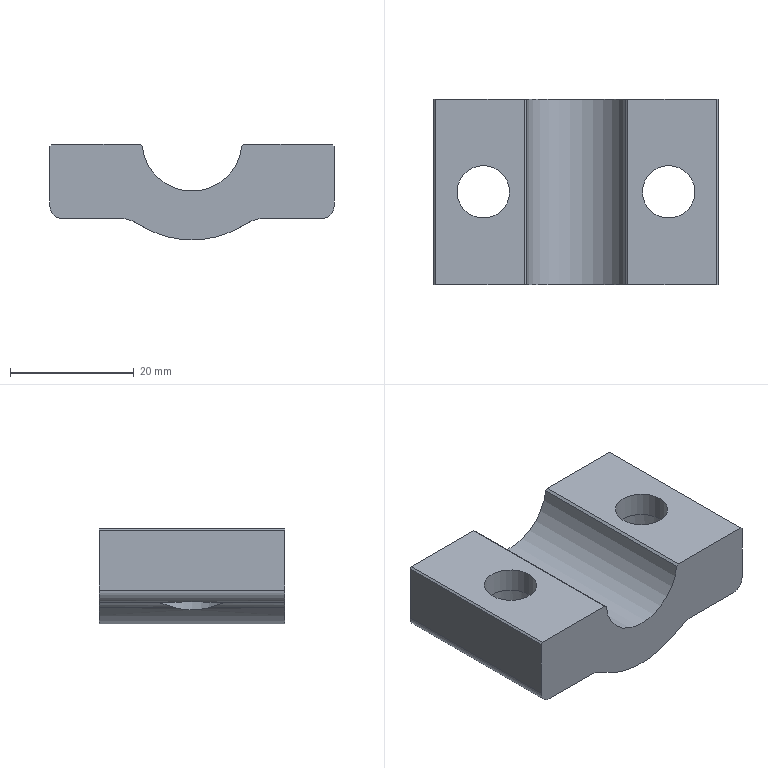NC program | NX | posted with a generic post | part box 46 x 30 x 15.5 mm
Lines 1 to 1684 of 1865, first 1555 of 1678 lines:
N10 G17 G21 G94 G90
(一刀光面 , TOOL : D50R6_1)
N12 T01 M6
N14 G54
N16 G17 G0 G90 X-52.998 Y-1.226 B0. C0. S2000 M3
N18 G43 Z30. H1
N20 Z3.
N22 G94 G1 Z0. F800.
N24 X-48. Y-1.08
N26 X48. Y1.739
N28 X52.998 Y1.886
N30 Z3.
N32 G0 Z30.
N34 M5
(ADAPTIVE_MILLING , TOOL : D10开粗_1)
N36 T02 M6
N38 G54
N40 G17 G0 G90 X-2.675 Y-20.135 B0. C0. S3000 M3
N42 G43 Z30. H2
N44 Z-28.
N46 G94 G1 X-2.599 Y-20.006 Z-28.937 F1500.
N48 X-2.522 Y-19.877 Z-29.308
N50 X-2.445 Y-19.748 Z-29.58
N52 X-2.369 Y-19.619 Z-29.8
N54 X-2.292 Y-19.49 Z-29.984
N56 X-2.216 Y-19.361 Z-30.142
N58 X-2.139 Y-19.232 Z-30.28
N60 X-2.063 Y-19.103 Z-30.4
N62 X-1.986 Y-18.974 Z-30.505
N64 X-1.91 Y-18.845 Z-30.598
N66 X-1.833 Y-18.716 Z-30.679
N68 X-1.757 Y-18.587 Z-30.75
N70 X-1.68 Y-18.458 Z-30.81
N72 X-1.604 Y-18.329 Z-30.862
N74 X-1.527 Y-18.2 Z-30.905
N76 X-1.451 Y-18.071 Z-30.939
N78 X-1.374 Y-17.942 Z-30.966
N80 X-1.298 Y-17.813 Z-30.985
N82 X-1.221 Y-17.684 Z-30.996
N84 X-1.145 Y-17.555 Z-31.
N86 X-0.452 Y-16.366
N88 G3 X-1.393 Y-14.946 R1.054
N90 X-5.461 Y-14.719 R28.472
N92 G1 X-23.555 Y-14.693
N94 G2 X-27.866 Y-12.146 R5.722
N96 X-29.421 Y-7.809 R9.762
N98 X-29.69 Y-2.044 R46.879
N100 G1 X-29.688 Y8.655
N102 G2 X-27.068 Y12.921 R5.762
N104 X-22.704 Y14.435 R9.932
N106 X-17.088 Y14.689 R48.084
N108 G1 X23.642 Y14.688
N110 G2 X27.877 Y12.131 R5.747
N112 X29.409 Y7.89 R9.699
N114 X29.686 Y2.539 R42.332
N116 X29.68 Y-8.741 R523.918
N118 X26.991 Y-12.972 R5.804
N120 X22.66 Y-14.441 R10.053
N122 X17.006 Y-14.69 R49.412
N124 G1 X0.569 Y-14.692
N126 G3 X-11.106 Y-14.4 R163.168
N128 G2 X-22.167 Y-14.38 R687.333
N130 X-27.657 Y-10.843 R6.986
N132 X-29.116 Y-6.184 R11.92
N134 X-29.391 Y0.294 R57.694
N136 X-29.38 Y7.166 R327.722
N138 X-25.778 Y12.695 R6.998
N140 X-20.997 Y14.138 R12.202
N142 X-14.706 Y14.391 R60.559
N144 G1 X21.829 Y14.396
N146 G2 X27.656 Y10.844 R6.967
N148 X29.115 Y6.184 R11.92
N150 X29.388 Y0.156 R54.035
N152 X29.38 Y-7.166 R332.394
N154 X25.811 Y-12.676 R6.993
N156 X21.184 Y-14.116 R11.962
N158 X14.856 Y-14.39 R56.43
N160 X0.746 Y-14.37 R762.628
N162 G3 X-11.706 Y-14.1 R214.037
N164 G2 X-20.854 Y-14.08 R721.079
N166 X-27.421 Y-9.795 R7.821
N168 X-28.832 Y-4.768 R13.795
N170 X-29.09 Y1.824 R66.58
N172 X-29.056 Y6.173 R66.922
N174 X-26.433 Y11.301 R7.585
N176 G1 X-26.341 Y11.392
N178 X-25.56 Y12.033
N180 G2 X-20.593 Y13.734 R12.355
N182 X-14.42 Y14.08 R48.356
N184 G1 X-9.433 Y14.099
N186 X20.142 Y14.098
N188 G2 X26.365 Y11.368 R7.784
N190 G1 X26.642 Y11.091
N192 X27.283 Y10.31
N194 X27.758 Y9.419
N196 G2 X28.907 Y4.167 R16.901
N198 X29.098 Y-4.116 R114.084
N200 X28.917 Y-7.104 R14.147
N202 X24.671 Y-12.486 R7.89
N204 X19.744 Y-13.835 R13.983
N206 X12.89 Y-14.092 R69.499
N208 X0.99 Y-14.06 R533.296
N210 G3 X-15.676 Y-13.798 R347.698
N212 G2 X-20.1 Y-13.754 R73.458
N214 X-27.142 Y-8.934 R8.455
N216 X-28.529 Y-3.707 R15.147
N218 X-28.753 Y5.06 R74.456
N220 X-28.115 Y7.864 R10.459
N222 G1 X-28.1 Y7.957
N224 X-28.051 Y8.456
N226 G2 X-27.281 Y10.312 R5.993
N228 X-26.429 Y11.304 R11.794
N230 G1 X-26.341 Y11.392
N232 X-25.56 Y12.033
N234 X-24.669 Y12.508
N236 X-23.703 Y12.801
N238 G2 X-15.324 Y13.747 R39.034
N240 X-6.737 Y13.799 R327.037
N242 G1 X18.701 Y13.798
N244 G2 X23.432 Y12.845 R10.105
N246 G1 X23.612 Y12.81
N248 G2 X24.672 Y12.507 R12.961
N250 X26.369 Y11.365 R5.971
N252 G3 X27.787 Y11.368 R1.003
N254 X27.787 Y12.782 R1.003
N256 G1 X26.533 Y14.326 Z-30.9
N258 X25.689 Y15.364 F15000.
N260 X25.589 Y15.471
N262 X25.474 Y15.561
N264 X25.347 Y15.634
N266 X25.21 Y15.688
N268 X24.023 Y16.057
N270 X23.547 Y16.197
N272 X23.066 Y16.321
N274 X22.582 Y16.43
N276 X22.094 Y16.522
N278 X21.604 Y16.599
N280 X20.988 Y16.675
N282 X20.37 Y16.728
N284 X19.75 Y16.76
N286 X19.13 Y16.769
N288 X-21.465 Y16.678
N290 X-21.6 Y16.668
N292 X-21.732 Y16.641
N294 X-21.859 Y16.596
N296 X-21.979 Y16.534
N298 X-22.09 Y16.457
N300 X-23.487 Y15.333
N302 X-24.524 Y14.488 Z-30.967 F1500.
N304 X-24.678 Y14.278 Z-30.98
N306 X-24.772 Y14.036 Z-30.993
N308 X-24.795 Y13.908 Z-31.
N310 X-24.801 Y13.76
N312 G3 X-23.703 Y12.801 R1.
N314 G1 X-22.699 Y12.9
N316 G2 X-16.524 Y13.388 R122.432
N318 X-6.626 Y13.499 R238.027
N320 G1 X17.479 Y13.498
N322 G2 X22.03 Y12.91 R15.267
N324 G1 X22.163 Y12.9
N326 X22.701
N328 X23.634 Y12.808
N330 G3 X24.702 Y14.047 R1.
N332 G1 X24.591 Y14.315 Z-30.985
N334 X24.407 Y14.54 Z-30.971
N336 X23.249 Y15.339 Z-30.9
N338 X22.235 Y16.027 F15000.
N340 X22.106 Y16.101
N342 X21.968 Y16.155
N344 X21.823 Y16.188
N346 X21.675 Y16.2
N348 X-20.741 Y16.292
N350 X-20.865 Y16.284
N352 X-20.987 Y16.262
N354 X-21.105 Y16.224
N356 X-21.218 Y16.172
N358 X-21.323 Y16.107
N360 X-22.321 Y15.396
N362 X-23.384 Y14.629 Z-30.966 F1500.
N364 X-23.554 Y14.419 Z-30.98
N366 X-23.662 Y14.171 Z-30.993
N368 X-23.69 Y14.038 Z-31.
N370 X-23.699 Y13.896
N372 G3 X-22.699 Y12.9 R1.
N374 G1 X-20.787
N376 G2 X-5.133 Y13.198 R277.211
N378 G1 X16.242
N380 G2 X20.329 Y12.9 R22.152
N382 G1 X22.167
N384 G3 X22.48 Y14.85 R1.
N386 G1 X20.563 Y15.383 Z-30.9
N388 X19.665 Y15.633 F15000.
N390 X19.533 Y15.66
N392 X19.397 Y15.669
N394 X-18.017
N396 X-18.152 Y15.66
N398 X-18.285 Y15.633
N400 X-19.158 Y15.39
N402 X-21.075 Y14.858 Z-31. F1500.
N404 G3 X-20.787 Y12.9 R1.
N406 G1 X-8.389
N408 X8.386
N410 X8.391
N412 X20.353
N414 G3 X21.453 Y14. R1.1
N416 X20.353 Y15.1 R1.1
N418 G1 X8.393 Y15.098
N420 X6.403 Z-30.9
N422 X-6.368 Y15.096 F15000.
N424 X-8.357 Y15.093 Z-31. F1500.
N426 G3 X-8.389 Y12.9 R1.1
N428 G1 X-7.446 Y12.813
N430 G3 X-2.884 Y12.611 R38.96
N432 X6.716 Y12.613 R688.468
N434 G1 X6.832 Y12.639
N436 X7.449 Y12.813
N438 X8.391 Y12.9
N440 G3 X8.328 Y15.095 R1.1
N442 G1 X6.338 Y15.08 Z-30.9
N444 X-5.963 Y14.981 F15000.
N446 X-7.314 Y14.958 Z-30.968 F1500.
N448 X-7.618 Y14.865 Z-30.984
N450 X-7.882 Y14.689 Z-31.
N452 G3 X-7.446 Y12.813 R1.1
N454 G1 X-7.014 Y12.69
N456 G3 X-3.381 Y12.353 R19.2
N458 X5.761 Y12.316 R248.059
N460 X6.292 Y12.433 R1.24
N462 G1 X6.539 Y12.556
N464 X6.863 Y12.647
N466 G3 X7.393 Y14.429 R1.1
N468 G1 X7.158 Y14.632 Z-30.984
N470 X6.875 Y14.761 Z-30.969
N472 X6.567 Y14.806 Z-30.953
N474 X5.514 Y14.809 Z-30.9
N476 X-5.579 Y14.845 F15000.
N478 X-6.853 Y14.839 Z-30.964 F1500.
N480 X-7.129 Y14.767 Z-30.978
N482 X-7.377 Y14.626 Z-30.993
N484 X-7.485 Y14.532 Z-31.
N486 X-7.586 Y14.418
N488 G3 X-7.014 Y12.69 R1.1
N490 G1 X-6.536 Y12.555
N492 G3 X-3.407 Y12.111 R12.813
N494 X5.064 Y12.033 R126.648
N496 X5.763 Y12.171 R1.657
N498 G1 X6.301 Y12.438
N500 G3 X6.746 Y14.006 R1.1
N502 G1 X6.543 Y14.246 Z-30.984
N504 X6.281 Y14.419 Z-30.968
N506 X5.98 Y14.511 Z-30.952
N508 X4.937 Y14.532 Z-30.9
N510 X-5.115 Y14.631 F15000.
N512 X-6.189 Z-30.954 F1500.
N514 X-6.482 Y14.551 Z-30.969
N516 X-6.742 Y14.393 Z-30.985
N518 X-6.949 Y14.17 Z-31.
N520 G3 X-6.536 Y12.555 R1.1
N522 G1 X-6.301 Y12.438
N524 G3 X-3.478 Y11.89 R9.865
N526 X4.495 Y11.754 R77.735
N528 X5.549 Y12.03 R2.077
N530 G1 X5.691 Y12.136
N532 X5.791 Y12.186
N534 G3 X6.262 Y13.711 R1.1
N536 G1 X6.092 Y13.938 Z-30.986
N538 X5.869 Y14.115 Z-30.971
N540 X5.609 Y14.228 Z-30.957
N542 X5.328 Y14.271 Z-30.943
N544 X4.478 Y14.29 Z-30.9
N546 X-4.856 Y14.502 F15000.
N548 X-5.938 Y14.516 Z-30.954 F1500.
N550 X-6.23 Y14.441 Z-30.97
N552 X-6.49 Y14.29 Z-30.985
N554 X-6.7 Y14.073 Z-31.
N556 G3 X-6.301 Y12.438 R1.1
N558 G1 X-5.898 Y12.238
N560 G3 X-2.979 Y11.627 R10.034
N562 X4.013 Y11.481 R53.438
N564 X5.215 Y11.781 R2.627
N566 G1 X5.251 Y11.806
N568 X5.551 Y12.031
N570 G3 X5.861 Y13.428 R1.1
N572 G1 X5.693 Y13.663 Z-30.985
N574 X5.471 Y13.845 Z-30.971
N576 X5.208 Y13.964 Z-30.956
N578 X4.924 Y14.01 Z-30.942
N580 X4.09 Y14.035 Z-30.9
N582 X-4.465 Y14.295 F15000.
N584 X-5.53 Y14.317 Z-30.954 F1500.
N586 X-5.827 Y14.241 Z-30.969
N588 X-6.092 Y14.086 Z-30.985
N590 X-6.304 Y13.863 Z-31.
N592 G3 X-5.898 Y12.238 R1.1
N594 G1 X-5.688 Y12.134
N596 G3 X-3.356 Y11.468 R6.927
N598 X3.607 Y11.215 R37.805
N600 X4.884 Y11.532 R2.908
N602 G1 X4.933 Y11.567
N604 X5.263 Y11.815
N606 G3 X5.575 Y13.21 R1.1
N608 G1 X5.408 Y13.445 Z-30.985
N610 X5.186 Y13.628 Z-30.971
N612 X4.924 Y13.747 Z-30.956
N614 X4.64 Y13.794 Z-30.942
N616 X3.806 Y13.822 Z-30.9
N618 X-4.134 Y14.085 F15000.
N620 X-5.153 Y14.107 Z-30.951 F1500.
N622 X-5.464 Y14.024 Z-30.967
N624 X-5.738 Y13.854 Z-30.984
N626 X-5.951 Y13.612 Z-31.
N628 G3 X-5.688 Y12.134 R1.1
N630 G1 X-5.538 Y12.022
N632 G3 X-3.196 Y11.252 R6.403
N634 X3.384 Y10.97 R28.714
N636 X4.667 Y11.334 R2.802
N638 G1 X4.743 Y11.395
N640 X4.933 Y11.567
N642 X4.963 Y11.59
N644 G3 X5.281 Y12.972 R1.1
N646 G1 X5.118 Y13.209 Z-30.986
N648 X4.898 Y13.395 Z-30.971
N650 X4.638 Y13.517 Z-30.957
N652 X4.355 Y13.568 Z-30.942
N654 X3.52 Y13.608 Z-30.9
N656 X-3.968 Y13.96 F15000.
N658 X-4.987 Y13.996 Z-30.951 F1500.
N660 X-5.3 Y13.917 Z-30.968
N662 X-5.576 Y13.752 Z-30.984
N664 X-5.792 Y13.513 Z-31.
N666 G3 X-5.538 Y12.022 R1.1
N668 G1 X-5.268 Y11.819
N670 G3 X-2.768 Y10.985 R6.955
N672 X3.117 Y10.725 R23.466
N674 X4.416 Y11.098 R3.059
N676 G1 X4.576 Y11.239
N678 X4.604 Y11.269
N680 X4.77 Y11.42
N682 G3 X5.006 Y12.747 R1.1
N684 G1 X4.815 Y13.008 Z-30.984
N686 X4.556 Y13.202 Z-30.967
N688 X4.252 Y13.313 Z-30.951
N690 X3.239 Y13.379 Z-30.9
N692 X-3.691 Y13.751 F15000.
N694 X-4.71 Y13.794 Z-30.951 F1500.
N696 X-5.023 Y13.717 Z-30.968
N698 X-5.3 Y13.554 Z-30.984
N700 X-5.518 Y13.317 Z-31.
N702 G3 X-5.268 Y11.819 R1.1
N704 G1 X-4.999 Y11.616
N706 G3 X-2.544 Y10.75 R6.898
N708 X2.956 Y10.497 R19.039
N710 X4.263 Y10.918 R2.878
N712 G1 X4.382 Y11.027
N714 X4.585 Y11.248
N716 G3 X4.747 Y12.506 R1.1
N718 G1 X4.558 Y12.764 Z-30.984
N720 X4.302 Y12.957 Z-30.968
N722 X4.002 Y13.069 Z-30.952
N724 X2.981 Y13.144 Z-30.9
N726 X-3.412 Y13.541 F15000.
N728 X-4.431 Y13.592 Z-30.951 F1500.
N730 X-4.744 Y13.518 Z-30.968
N732 X-5.022 Y13.357 Z-30.984
N734 X-5.242 Y13.122 Z-31.
N736 G3 X-4.999 Y11.616 R1.1
N738 G1 X-4.932 Y11.566
N740 X-4.849 Y11.491
N742 G3 X-2.567 Y10.567 R5.905
N744 X2.79 Y10.274 R16.159
N746 X4.075 Y10.709 R2.832
N748 G1 X4.179 Y10.807
N750 X4.382 Y11.028
N752 G3 X4.538 Y12.297 R1.1
N754 G1 X4.35 Y12.549 Z-30.984
N756 X4.099 Y12.738 Z-30.968
N758 X3.804 Y12.847 Z-30.952
N760 X2.765 Y12.931 Z-30.9
N762 X-3.181 Y13.344 F15000.
N764 X-4.196 Y13.403 Z-30.951 F1500.
N766 X-4.511 Y13.331 Z-30.967
N768 X-4.791 Y13.17 Z-30.984
N770 X-5.012 Y12.935 Z-31.
N772 G3 X-4.849 Y11.491 R1.1
N774 G1 X-4.626 Y11.289
N776 G3 X-2.23 Y10.306 R6.145
N778 X2.794 Y10.086 R13.405
N780 X3.946 Y10.555 R2.253
N782 G1 X3.98 Y10.59
N784 X4.183 Y10.811
N786 G3 X4.341 Y12.077 R1.1
N788 G1 X4.155 Y12.329 Z-30.984
N790 X3.905 Y12.518 Z-30.968
N792 X3.612 Y12.629 Z-30.953
N794 X2.57 Y12.719 Z-30.9
N796 X-2.952 Y13.137 F15000.
N798 X-3.967 Y13.202 Z-30.951 F1500.
N800 X-4.282 Y13.132 Z-30.967
N802 X-4.563 Y12.973 Z-30.984
N804 X-4.786 Y12.739 Z-31.
N806 G3 X-4.527 Y11.185 R1.158
N808 X-2.363 Y10.159 R5.259
N810 X2.666 Y9.88 R11.9
N812 X3.824 Y10.389 R2.204
N814 X4.274 Y11.278 R1.578
N816 X4.148 Y11.857 R1.1
N818 G1 X3.963 Y12.109 Z-30.984
N820 X3.716 Y12.299 Z-30.969
N822 X3.424 Y12.412 Z-30.953
N824 X2.381 Y12.512 Z-30.9
N826 X-2.763 Y12.951 F15000.
N828 X-3.783 Y13.027 Z-30.951 F1500.
N830 X-4.097 Y12.961 Z-30.968
N832 X-4.379 Y12.807 Z-30.984
N834 X-4.604 Y12.578 Z-31.
N836 G3 X-4.527 Y11.185 R1.1
N838 G1 X-4.374 Y11.019
N840 G3 X-2.25 Y9.954 R5.158
N842 X2.604 Y9.694 R10.483
N844 X3.744 Y10.246 R2.135
N846 G1 X3.837 Y10.369
N848 X3.956 Y10.56
N850 G3 X3.984 Y11.68 R1.1
N852 G1 X3.801 Y11.922 Z-30.985
N854 X3.559 Y12.104 Z-30.969
N856 X3.277 Y12.214 Z-30.954
N858 X2.206 Y12.325 Z-30.9
N860 X-2.606 Y12.778 F15000.
N862 X-3.622 Y12.861 Z-30.951 F1500.
N864 X-3.938 Y12.797 Z-30.968
N866 X-4.221 Y12.645 Z-30.984
N868 X-4.448 Y12.417 Z-31.
N870 G3 X-4.374 Y11.019 R1.1
N872 G1 X-4.172 Y10.798
N874 G3 X-1.881 Y9.679 R5.381
N876 X2.528 Y9.51 R9.392
N878 X3.664 Y10.106 R2.044
N880 G1 X3.725 Y10.191
N882 X3.845 Y10.382
N884 G3 X3.855 Y11.531 R1.1
N886 G1 X3.672 Y11.761 Z-30.985
N888 X3.434 Y11.934 Z-30.97
N890 X3.158 Y12.037 Z-30.956
N892 X2.06 Y12.148 Z-30.9
N894 X-2.405 Y12.559 F15000.
N896 X-3.422 Y12.64 Z-30.951 F1500.
N898 X-3.737 Y12.576 Z-30.968
N900 X-4.02 Y12.423 Z-30.984
N902 X-4.247 Y12.194 Z-31.
N904 G3 X-4.172 Y10.798 R1.1
N906 G1 X-3.962 Y10.57
N908 G3 X-1.6 Y9.431 R5.475
N910 X2.558 Y9.36 R8.289
N912 X3.608 Y10.004 R1.785
N914 G1 X3.728 Y10.194
N916 G3 X3.716 Y11.379 R1.1
N918 G1 X3.526 Y11.599 Z-30.985
N920 X3.285 Y11.762 Z-30.971
N922 X3.01 Y11.857 Z-30.956
N924 X1.899 Y11.937 Z-30.9
N926 X-2.076 Y12.191 F15000.
N928 X-3.115 Y12.246 Z-30.952 F1500.
N930 X-3.422 Y12.176 Z-30.968
N932 X-3.697 Y12.022 Z-30.984
N934 X-3.917 Y11.796 Z-31.
N936 G3 X-3.617 Y10.212 R1.114
N938 X-0.637 Y9.054 R6.462
N940 X2.699 Y9.258 R6.944
N942 X3.491 Y9.816 R1.395
N944 G1 X3.61 Y10.006
N946 G3 X3.605 Y11.181 R1.1
N948 G1 X3.423 Y11.399 Z-30.986
N950 X3.191 Y11.562 Z-30.971
N952 X2.926 Y11.661 Z-30.957
N954 X1.796 Y11.782 Z-30.9
N956 X-2.055 Y12.162 F15000.
N958 X-3.081 Y12.252 Z-30.952 F1500.
N960 X-3.394 Y12.191 Z-30.968
N962 X-3.676 Y12.043 Z-30.984
N964 X-3.904 Y11.821 Z-31.
N966 G3 X-3.962 Y10.57 R1.1
N968 G1 X-3.863 Y10.411
N970 G3 X-1.993 Y9.222 R4.072
N972 X2.42 Y9.014 R7.269
N974 X3.574 Y9.97 R1.638
N976 X3.496 Y11.002 R1.1
N978 G1 X3.316 Y11.219 Z-30.986
N980 X3.086 Y11.383 Z-30.972
N982 X2.822 Y11.483 Z-30.957
N984 X1.689 Y11.612 Z-30.9
N986 X-1.927 Y11.994 F15000.
N988 X-2.971 Y12.093 Z-30.953 F1500.
N990 X-3.278 Y12.037 Z-30.968
N992 X-3.558 Y11.897 Z-30.984
N994 X-3.786 Y11.684 Z-31.
N996 G3 X-3.863 Y10.411 R1.1
N998 G1 X-3.764 Y10.252
N1000 G3 X-1.914 Y9.039 R4.047
N1002 X2.313 Y8.833 R6.919
N1004 X3.354 Y9.528 R1.746
N1006 X3.362 Y10.771 R1.169
N1008 G1 X3.152 Y11.01 Z-30.984
N1010 X2.882 Y11.179 Z-30.968
N1012 X2.576 Y11.264 Z-30.952
N1014 X1.552 Y11.393 Z-30.9
N1016 X-1.8 Y11.814 F15000.
N1018 X-2.849 Y11.935 Z-30.953 F1500.
N1020 X-3.155 Y11.886 Z-30.969
N1022 X-3.436 Y11.754 Z-30.984
N1024 X-3.668 Y11.548 Z-31.
N1026 G3 X-3.764 Y10.252 R1.1
N1028 G1 X-3.664 Y10.093
N1030 G3 X-1.799 Y8.846 R3.942
N1032 X2.248 Y8.668 R6.552
N1034 X3.294 Y9.376 R1.801
N1036 G1 X3.359 Y9.509
N1038 X3.428 Y9.683
N1040 G3 X3.314 Y10.704 R1.1
N1042 G1 X3.102 Y10.936 Z-30.984
N1044 X2.834 Y11.099 Z-30.968
N1046 X2.53 Y11.179 Z-30.952
N1048 X1.493 Y11.298 Z-30.9
N1050 X-1.707 Y11.666 F15000.
N1052 X-2.761 Y11.776 Z-30.953 F1500.
N1054 X-3.065 Y11.724 Z-30.969
N1056 X-3.344 Y11.59 Z-30.984
N1058 X-3.574 Y11.384 Z-31.
N1060 G3 X-3.664 Y10.093 R1.1
N1062 G1 X-3.545 Y9.902
N1064 G3 X-1.65 Y8.643 R3.964
N1066 X2.239 Y8.524 R6.144
N1068 X3.249 Y9.249 R1.738
N1070 G1 X3.3 Y9.358
N1072 X3.369 Y9.533
N1074 G3 X3.235 Y10.582 R1.1
N1076 G1 X3.024 Y10.801 Z-30.985
N1078 X2.761 Y10.954 Z-30.969
N1080 X2.466 Y11.029 Z-30.954
N1082 X1.399 Y11.147 Z-30.9
N1084 X-1.59 Y11.479 F15000.
N1086 X-2.645 Y11.585 Z-30.953 F1500.
N1088 X-2.949 Y11.532 Z-30.969
N1090 X-3.227 Y11.397 Z-30.984
N1092 X-3.456 Y11.191 Z-31.
N1094 G3 X-3.545 Y9.902 R1.1
N1096 G1 X-3.461 Y9.768
N1098 G3 X-1.724 Y8.524 R3.589
N1100 X2.338 Y8.427 R5.681
N1102 X3.237 Y9.197 R1.514
N1104 G1 X3.305 Y9.371
N1106 G3 X3.151 Y10.449 R1.1
N1108 G1 X2.934 Y10.66 Z-30.985
N1110 X2.669 Y10.804 Z-30.97
N1112 X2.374 Y10.87 Z-30.954
N1114 X1.298 Y10.96 Z-30.9
N1116 X-1.408 Y11.187 F15000.
N1118 X-2.495 Y11.268 Z-30.955 F1500.
N1120 X-2.788 Y11.212 Z-30.97
N1122 X-3.056 Y11.079 Z-30.985
N1124 X-3.278 Y10.879 Z-31.
N1126 G3 X-3.082 Y9.238 R1.175
N1128 X0.036 Y7.967 R5.119
N1130 X2.637 Y8.451 R4.489
N1132 X3.174 Y9.037 R1.168
N1134 G1 X3.242 Y9.212
N1136 G3 X3.084 Y10.293 R1.1
N1138 G1 X2.877 Y10.496 Z-30.985
N1140 X2.623 Y10.637 Z-30.971
N1142 X2.341 Y10.707 Z-30.956
N1144 X1.233 Y10.832 Z-30.9
N1146 X-1.369 Y11.124 F15000.
N1148 X-2.451 Y11.235 Z-30.955 F1500.
N1150 X-2.746 Y11.187 Z-30.97
N1152 X-3.018 Y11.061 Z-30.985
N1154 X-3.246 Y10.866 Z-31.
N1156 G3 X-3.151 Y9.229 R1.221
N1158 X-0.576 Y7.897 R4.532
N1160 X2.452 Y8.222 R4.845
N1162 X3.115 Y8.887 R1.24
N1164 G1 X3.183 Y9.061
N1166 G3 X3.017 Y10.153 R1.1
N1168 G1 X2.812 Y10.35 Z-30.986
N1170 X2.563 Y10.487 Z-30.971
N1172 X2.288 Y10.556 Z-30.957
N1174 X1.16 Y10.689 Z-30.9
N1176 X-1.29 Y10.976 F15000.
N1178 X-2.388 Y11.095 Z-30.956 F1500.
N1180 X-2.678 Y11.051 Z-30.97
N1182 X-2.947 Y10.931 Z-30.985
N1184 X-3.174 Y10.745 Z-31.
N1186 G3 X-3.189 Y9.203 R1.197
N1188 X-0.822 Y7.802 R4.112
N1190 X2.356 Y8.048 R4.82
N1192 X3.11 Y9.764 R1.351
N1194 G1 X2.96 Y10.01
N1196 X2.756 Y10.205 Z-30.986
N1198 X2.509 Y10.342 Z-30.972
N1200 X2.236 Y10.412 Z-30.957
N1202 X1.104 Y10.549 Z-30.9
N1204 X-1.217 Y10.831 F15000.
N1206 X-2.326 Y10.956 Z-30.956 F1500.
N1208 X-2.613 Y10.914 Z-30.971
N1210 X-2.879 Y10.799 Z-30.985
N1212 X-3.106 Y10.619 Z-31.
N1214 G3 X-3.138 Y9.062 R1.206
N1216 X-0.788 Y7.65 R4.016
N1218 X2.368 Y7.932 R4.605
N1220 X2.976 Y9.66 R1.241
N1222 G1 X2.883 Y9.791
N1224 X2.643 Y10.008 Z-30.984
N1226 X2.351 Y10.145 Z-30.967
N1228 X1.026 Y10.35 Z-30.9
N1230 X-1.134 Y10.664 F15000.
N1232 X-2.245 Y10.816 Z-30.956 F1500.
N1234 X-2.531 Y10.782 Z-30.971
N1236 X-2.799 Y10.675 Z-30.985
N1238 X-3.03 Y10.501 Z-31.
N1240 G3 X-3.283 Y9.314 R1.1
N1242 G1 X-3.214 Y9.139
N1244 G3 X-1.49 Y7.734 R3.246
N1246 X2.148 Y7.698 R4.798
N1248 X3.066 Y8.638 R1.49
N1250 G1 X3.075 Y8.675
N1252 X3.103 Y8.823
N1254 G3 X2.859 Y9.742 R1.1
N1256 G1 X2.658 Y9.925 Z-30.986
N1258 X2.419 Y10.054 Z-30.973
N1260 X2.155 Y10.119 Z-30.959
N1262 X0.992 Y10.262 Z-30.9
N1264 X-1.075 Y10.514 F15000.
N1266 X-2.199 Y10.642 Z-30.957 F1500.
N1268 X-2.482 Y10.602 Z-30.971
N1270 X-2.744 Y10.492 Z-30.986
N1272 X-2.97 Y10.318 Z-31.
N1274 G3 X-3.014 Y8.743 R1.211
N1276 X-0.667 Y7.34 R3.913
N1278 X2.422 Y7.727 R4.201
N1280 X3.05 Y8.545 R1.214
N1282 G1 X3.078 Y8.692
N1284 G3 X2.817 Y9.63 R1.1
N1286 G1 X2.575 Y9.833 Z-30.984
N1288 X2.286 Y9.959 Z-30.968
N1290 X0.942 Y10.134 Z-30.9
N1292 X-1.02 Y10.374 F15000.
N1294 X-2.144 Y10.502 Z-30.957 F1500.
N1296 X-2.427 Y10.463 Z-30.971
N1298 X-2.689 Y10.353 Z-30.986
N1300 X-2.915 Y10.178 Z-31.
N1302 G3 X-3.037 Y8.72 R1.193
N1304 X-1.129 Y7.331 R3.462
N1306 X2.247 Y7.504 R4.385
N1308 X3.025 Y8.415 R1.386
N1310 G1 X3.053 Y8.563
N1312 G3 X2.767 Y9.529 R1.1
N1314 G1 X2.519 Y9.722 Z-30.984
N1316 X2.227 Y9.838 Z-30.968
N1318 X0.875 Y9.971 Z-30.9
N1320 X-0.927 Y10.133 F15000.
N1322 X-2.104 Y10.227 Z-30.959 F1500.
N1324 X-2.42 Y10.162 Z-30.976
N1326 X-2.703 Y10.008 Z-30.992
N1328 X-2.824 Y9.902 Z-31.
N1330 X-2.926 Y9.783
N1332 G3 X-2.818 Y8.317 R1.159
N1334 X0.039 Y6.957 R4.122
N1336 X2.548 Y7.587 R3.7
N1338 X2.996 Y8.265 R1.131
N1340 G1 X3.013 Y8.35
N1342 X3.027 Y8.424
N1344 G3 X2.729 Y9.402 R1.1
N1346 G1 X2.494 Y9.583 Z-30.985
N1348 X2.219 Y9.694 Z-30.97
N1350 X0.836 Y9.865 Z-30.9
N1352 X-0.899 Y10.067 F15000.
N1354 X-2.069 Y10.191 Z-30.959 F1500.
N1356 X-2.388 Y10.133 Z-30.976
N1358 X-2.676 Y9.985 Z-30.992
N1360 X-2.8 Y9.881 Z-31.
N1362 X-2.903 Y9.766
N1364 G3 X-2.823 Y8.23 R1.262
N1366 X-0.073 Y6.834 R3.957
N1368 X2.549 Y7.474 R3.651
N1370 X2.964 Y8.113 R1.125
N1372 G1 X3.002 Y8.297
N1374 G3 X2.694 Y9.306 R1.1
N1376 G1 X2.463 Y9.479 Z-30.985
N1378 X2.195 Y9.586 Z-30.971
N1380 X0.795 Y9.76 Z-30.9
N1382 X-0.856 Y9.953 F15000.
N1384 X-2.044 Y10.081 Z-30.96 F1500.
N1386 X-2.356 Y10.026 Z-30.976
N1388 X-2.64 Y9.885 Z-30.992
N1390 X-2.763 Y9.786 Z-31.
N1392 X-2.871 Y9.67
N1394 G3 X-2.806 Y8.113 R1.28
N1396 X-0.09 Y6.703 R3.888
N1398 X2.557 Y7.368 R3.569
N1400 X2.936 Y7.978 R1.083
N1402 G1 X2.967 Y8.125
N1404 G3 X2.652 Y9.141 R1.1
N1406 G1 X2.429 Y9.307 Z-30.986
N1408 X2.172 Y9.411 Z-30.972
N1410 X0.753 Y9.611 Z-30.9
N1412 X-0.802 Y9.82 F15000.
N1414 X-2.001 Y9.971 Z-30.961 F1500.
N1416 X-2.309 Y9.924 Z-30.976
N1418 X-2.591 Y9.793 Z-30.992
N1420 X-2.716 Y9.699 Z-31.
N1422 X-2.817 Y9.598
N1424 G3 X-3.073 Y8.666 R1.1
N1426 G1 X-3.045 Y8.518
N1428 G3 X-1.737 Y7.084 R2.616
N1430 X2.151 Y6.971 R4.184
N1432 X2.906 Y7.833 R1.375
N1434 G1 X2.937 Y7.98
N1436 G3 X2.612 Y9.005 R1.1
N1438 G1 X2.393 Y9.164 Z-30.986
N1440 X2.141 Y9.266 Z-30.973
N1442 X0.71 Y9.469 Z-30.9
N1444 X-0.754 Y9.669 F15000.
N1446 X-1.968 Y9.823 Z-30.962 F1500.
N1448 X-2.27 Y9.78 Z-30.977
N1450 X-2.549 Y9.655 Z-30.992
N1452 X-2.672 Y9.565 Z-31.
N1454 X-2.777 Y9.464
N1456 G3 X-2.765 Y7.859 R1.257
N1458 X0.072 Y6.429 R3.822
N1460 X2.565 Y7.152 R3.398
N1462 X2.874 Y7.685 R1.079
N1464 G1 X2.901 Y7.807
N1466 X2.909 Y7.844
N1468 G3 X2.58 Y8.873 R1.1
N1470 G1 X2.365 Y9.029 Z-30.987
N1472 X2.119 Y9.129 Z-30.973
N1474 X0.678 Y9.345 Z-30.9
N1476 X-0.718 Y9.547 F15000.
N1478 X-1.937 Y9.713 Z-30.962 F1500.
N1480 X-2.237 Y9.673 Z-30.977
N1482 X-2.515 Y9.553 Z-30.992
N1484 X-2.638 Y9.465 Z-31.
N1486 X-2.746 Y9.364
N1488 G3 X-3.024 Y8.408 R1.1
N1490 G1 X-3.01 Y8.334
N1492 X-2.995 Y8.26
N1494 G3 X-1.708 Y6.823 R2.564
N1496 X2.111 Y6.71 R4.091
N1498 X2.841 Y7.54 R1.37
N1500 G1 X2.874 Y7.686
N1502 G3 X2.55 Y8.732 R1.1
N1504 G1 X2.337 Y8.887 Z-30.987
N1506 X2.093 Y8.987 Z-30.973
N1508 X0.65 Y9.211 Z-30.9
N1510 X-0.677 Y9.41 F15000.
N1512 X-1.904 Y9.583 Z-30.962 F1500.
N1514 X-2.2 Y9.546 Z-30.977
N1516 X-2.476 Y9.431 Z-30.992
N1518 X-2.6 Y9.346 Z-31.
N1520 X-2.712 Y9.244
N1522 G3 X-2.78 Y7.689 R1.262
N1524 X-0.194 Y6.199 R3.596
N1526 X2.383 Y6.777 R3.548
N1528 X2.497 Y8.466 R1.097
N1530 G1 X2.245 Y8.64 Z-30.985
N1532 X1.954 Y8.736 Z-30.969
N1534 X0.601 Y8.98 Z-30.9
N1536 X-0.632 Y9.202 F15000.
N1538 X-1.861 Y9.413 Z-30.963 F1500.
N1540 X-2.156 Y9.384 Z-30.978
N1542 X-2.432 Y9.277 Z-30.993
N1544 X-2.556 Y9.196 Z-31.
N1546 X-2.671 Y9.096
N1548 G3 X-2.741 Y7.534 R1.239
N1550 X-0.124 Y6.065 R3.584
N1552 X2.419 Y6.699 R3.421
N1554 X2.645 Y6.992 R1.139
N1556 X2.846 Y7.562 R1.731
N1558 X2.519 Y8.611 R1.1
N1560 G1 X2.29 Y8.773 Z-30.986
N1562 X2.028 Y8.873 Z-30.972
N1564 X0.61 Y9.033 Z-30.9
N1566 X-0.626 Y9.164 F15000.
N1568 X-1.885 Y9.289 Z-30.964 F1500.
N1570 X-2.17 Y9.244 Z-30.978
N1572 X-2.434 Y9.126 Z-30.993
N1574 X-2.551 Y9.042 Z-31.
N1576 X-2.661 Y8.94
N1578 G3 X-2.934 Y7.967 R1.1
N1580 G1 X-2.901 Y7.807
N1582 G3 X-1.548 Y6.373 R2.668
N1584 X2.084 Y6.347 R3.905
N1586 X2.551 Y6.806 R1.175
N1588 G1 X2.652 Y7.007
N1590 G3 X2.448 Y8.278 R1.1
N1592 G1 X2.227 Y8.45 Z-30.986
N1594 X1.97 Y8.56 Z-30.972
N1596 X0.559 Y8.781 Z-30.9
N1598 X-0.578 Y8.952 F15000.
N1600 X-1.808 Y9.126 Z-30.962 F1500.
N1602 X-2.104 Y9.09 Z-30.977
N1604 X-2.379 Y8.975 Z-30.992
N1606 X-2.502 Y8.891 Z-31.
N1608 X-2.615 Y8.789
N1610 G3 X-2.901 Y7.807 R1.1
N1612 G1 X-2.867 Y7.656
N1614 G3 X-1.4 Y6.179 R2.688
N1616 X2.072 Y6.231 R3.787
N1618 X2.346 Y7.882 R1.125
N1620 G1 X2.13 Y8.083 Z-30.985
N1622 X1.869 Y8.219 Z-30.97
N1624 X0.505 Y8.524 Z-30.9
N1626 X-0.536 Y8.75 F15000.
N1628 X-1.716 Y8.994 Z-30.961 F1500.
N1630 X-2.028 Y8.971 Z-30.976
N1632 X-2.321 Y8.862 Z-30.992
N1634 X-2.452 Y8.777 Z-31.
N1636 X-2.572 Y8.674
N1638 G3 X-2.655 Y7.123 R1.227
N1640 X-0.016 Y5.682 R3.501
N1642 X1.948 Y6.065 R3.234
N1644 X2.225 Y7.486 R1.07
N1646 G1 X2.055 Y7.697 Z-30.986
N1648 X1.837 Y7.859 Z-30.973
N1650 X1.586 Y7.96 Z-30.959
N1652 X0.45 Y8.259 Z-30.9
N1654 X-0.483 Y8.504 F15000.
N1656 X-1.67 Y8.805 Z-30.962 F1500.
N1658 X-1.975 Y8.796 Z-30.977
N1660 X-2.264 Y8.702 Z-30.992
N1662 X-2.396 Y8.624 Z-31.
N1664 X-2.52 Y8.525
N1666 G3 X-2.834 Y7.509 R1.069
N1668 X-2.688 Y7.077 R1.385
N1670 X-0.173 Y5.577 R3.383
N1672 X1.579 Y5.787 R3.176
N1674 X2.058 Y7.128 R1.1
N1676 G1 X1.923 Y7.381 Z-30.986
N1678 X1.727 Y7.59 Z-30.971
N1680 X1.484 Y7.741 Z-30.957
N1682 X0.409 Y8.078 Z-30.9
N1684 X-0.449 Y8.339 F15000.
N1686 X-1.525 Y8.657 Z-30.956 F1500.
N1688 X-1.813 Y8.666 Z-30.971
N1690 X-2.094 Y8.6 Z-30.985
N1692 X-2.348 Y8.464 Z-31.
N1694 G3 X-2.688 Y7.077 R1.1
N1696 G1 X-2.57 Y6.843
N1698 G3 X-0.352 Y5.483 R3.233
N1700 X1.049 Y5.517 R3.008
N1702 X2.561 Y6.825 R2.746
N1704 X2.377 Y8.075 R1.1
N1706 G1 X2.147 Y8.261 Z-30.985
N1708 X1.877 Y8.378 Z-30.97
N1710 X1.584 Y8.419 Z-30.955
N1712 X0.483 Y8.425 Z-30.9
N1714 X-0.469 Y8.431 F15000.
N1716 X-1.727 Y8.428 Z-30.963 F1500.
N1718 X-2.008 Y8.353 Z-30.978
N1720 X-2.26 Y8.206 Z-30.993
N1722 X-2.37 Y8.109 Z-31.
N1724 X-2.469 Y7.994
N1726 G3 X-2.57 Y6.843 R1.1
N1728 X-2.152 Y6.262 R1.865
N1730 X0.218 Y5.328 R3.318
N1732 X1.053 Y5.518 R2.166
N1734 X1.682 Y6.935 R1.1
N1736 G1 X1.532 Y7.206 Z-30.984
N1738 X1.313 Y7.424 Z-30.969
N1740 X1.041 Y7.573 Z-30.953
N1742 X0.012 Y7.812 Z-30.9
N1744 X-0.166 Y7.851 F15000.
N1746 X-1.229 Y8.076 Z-30.955 F1500.
N1748 X-1.529 Y8.059 Z-30.97
N1750 X-1.812 Y7.963 Z-30.985
N1752 X-2.059 Y7.793 Z-31.
N1754 G3 X-2.152 Y6.262 R1.1
N1756 X0.228 Y5.329 R2.844
N1758 X1.095 Y6.467 R1.
N1760 G1 X1.077 Y6.558 Z-30.995
N1762 X1.051 Y6.648 Z-30.991
N1764 X0.463 Y8.352 Z-30.9
N1766 X0.207 Y9.097 F15000.
N1768 X0.169 Y9.237
N1770 X0.153 Y9.381
N1772 X0.157 Y9.525
N1774 X0.182 Y9.668
N1776 X0.228 Y9.805
N1778 X1.426 Y12.697
N1780 X1.542 Y12.949
N1782 X1.678 Y13.19
N1784 X1.833 Y13.419
N1786 X2.006 Y13.636
N1788 X2.195 Y13.838
N1790 X2.401 Y14.023
N1792 X2.62 Y14.192
N1794 X2.853 Y14.343
N1796 X3.096 Y14.474
N1798 X3.35 Y14.586
N1800 X4.301 Y14.959
N1802 X4.88 Y15.174
N1804 X5.466 Y15.367
N1806 X6.058 Y15.538
N1808 X6.657 Y15.687
N1810 X7.261 Y15.813
N1812 X7.869 Y15.917
N1814 X8.481 Y15.998
N1816 X9.095 Y16.056
N1818 X11.575 Y16.243
N1820 X12.675 Y16.316
N1822 X13.776 Y16.367
N1824 X14.878 Y16.396
N1826 X15.981 Y16.404
N1828 X17.083 Y16.391
N1830 X18.185 Y16.356
N1832 X19.286 Y16.3
N1834 X20.385 Y16.223
N1836 X21.483 Y16.124
N1838 X25.575 Y15.715
N1840 X25.863 Y15.676
N1842 X26.148 Y15.616
N1844 X26.427 Y15.536
N1846 X26.7 Y15.436
N1848 X26.965 Y15.317
N1850 X27.221 Y15.179
N1852 X27.466 Y15.024
N1854 X27.7 Y14.851
N1856 X27.92 Y14.662
N1858 X28.917 Y13.743
N1860 X29.018 Y13.636
N1862 X29.101 Y13.514
N1864 X29.166 Y13.382
N1866 X29.211 Y13.242
N1868 X29.235 Y13.097
N1870 X29.237 Y12.95
N1872 X29.218 Y12.804
N1874 X29.178 Y12.662
N1876 X29.117 Y12.528
N1878 X28.952 Y12.228
N1880 X27.838 Y10.189 Z-31. F1500.
N1882 G3 X27.758 Y9.419 R1.
N1884 G1 X28.051 Y8.453
N1886 X28.07 Y8.267
N1888 G2 X28.779 Y-1.389 R60.802
N1890 X28.727 Y-5.362 R41.26
N1892 X24.047 Y-12.084 R8.42
N1894 X18.83 Y-13.515 R14.843
N1896 X11.751 Y-13.79 R71.169
N1898 X-4.425 Y-13.579 R324.422
N1900 G3 X-18.378 Y-13.488 R819.5
N1902 G2 X-23.573 Y-12.016 R9.574
N1904 X-27.374 Y-6.891 R9.834
N1906 X-28.335 Y-1.479 R20.792
N1908 X-28.446 Y4.105 R60.805
N1910 X-28.15 Y6.229 R28.912
N1912 G1 Y7.451
N1914 X-28.098 Y7.973
N1916 G3 X-28.578 Y8.945 R1.046
N1918 G1 X-30.097 Y10.229 Z-30.9
N1920 X-30.275 Y10.379 F15000.
N1922 X-30.382 Y10.484
N1924 X-30.472 Y10.604
N1926 X-30.543 Y10.737
N1928 X-30.594 Y10.878
N1930 X-30.622 Y11.026
N1932 X-30.629 Y11.176
N1934 X-30.612 Y11.325
N1936 X-30.574 Y11.47
N1938 X-30.514 Y11.608
N1940 X-30.434 Y11.736
N1942 X-30.336 Y11.85
N1944 X-26.424 Y15.762
N1946 X-26.215 Y15.955
N1948 X-25.992 Y16.131
N1950 X-25.755 Y16.289
N1952 X-25.507 Y16.428
N1954 X-25.249 Y16.547
N1956 X-24.982 Y16.646
N1958 X-24.708 Y16.723
N1960 X-24.429 Y16.779
N1962 X-24.147 Y16.812
N1964 X-23.863 Y16.823
N1966 X18.509
N1968 X19.179 Y16.813
N1970 X19.848 Y16.783
N1972 X20.517 Y16.732
N1974 X21.183 Y16.662
N1976 X21.847 Y16.571
N1978 X22.508 Y16.461
N1980 X23.165 Y16.331
N1982 X23.818 Y16.181
N1984 X24.467 Y16.011
N1986 X25.11 Y15.822
N1988 X26.745 Y15.314
N1990 X27.049 Y15.209
N1992 X27.346 Y15.085
N1994 X27.634 Y14.943
N1996 X27.912 Y14.782
N1998 X28.18 Y14.604
N2000 X28.435 Y14.41
N2002 X28.678 Y14.199
N2004 X28.908 Y13.974
N2006 X29.122 Y13.735
N2008 X29.321 Y13.482
N2010 X30.308 Y12.143
N2012 X30.385 Y12.021
N2014 X30.443 Y11.889
N2016 X30.482 Y11.751
N2018 X30.501 Y11.608
N2020 X30.499 Y11.464
N2022 X30.476 Y11.321
N2024 X30.433 Y11.184
N2026 X30.371 Y11.054
N2028 X30.29 Y10.934
N2030 X30.194 Y10.827
N2032 X29.967 Y10.61
N2034 X28.374 Y9.087 Z-31. F1500.
N2036 G3 X28.07 Y8.267 R1.
N2038 G1 X28.15 Y7.449
N2040 Y6.699
N2042 G2 X28.487 Y-2.8 R204.818
N2044 X27.714 Y-7.274 R10.954
N2046 X22.836 Y-12.003 R9.204
N2048 X17.337 Y-13.267 R17.486
N2050 X9.655 Y-13.494 R96.426
N2052 X-4.606 Y-13.28 R341.727
N2054 G3 X-17.404 Y-13.187 R594.542
N2056 G2 X-22.295 Y-12.079 R10.8
N2058 X-26.775 Y-6.965 R9.811
N2060 G1 X-27.193 Y-5.823
N2062 X-27.719 Y-4.694
N2064 X-28.041 Y-3.49
N2066 X-28.15 Y-2.249
N2068 Y6.233
N2070 G3 X-29.25 Y7.333 R1.1
N2072 X-30.35 Y6.233 R1.1
N2074 G1 Y0.863
N2076 G3 X-29.25 Y-0.237 R1.1
N2078 X-28.15 Y0.863 R1.1
N2080 G1 Y2.813
N2082 G3 X-28.599 Y3.648 R1.
N2084 G1 X-28.973 Y3.894
N2086 X-30.633 Y4.99 Z-30.9
N2088 X-30.866 Y5.144 F15000.
N2090 X-30.978 Y5.229
N2092 X-31.076 Y5.33
N2094 X-31.16 Y5.443
N2096 X-31.227 Y5.568
N2098 X-31.276 Y5.7
N2100 X-31.305 Y5.838
N2102 X-31.315 Y5.978
N2104 Y9.452
N2106 X-31.304 Y9.736
N2108 X-31.27 Y10.018
N2110 X-31.215 Y10.297
N2112 X-31.138 Y10.571
N2114 X-31.039 Y10.838
N2116 X-30.92 Y11.096
N2118 X-30.781 Y11.344
N2120 X-30.623 Y11.58
N2122 X-30.447 Y11.804
N2124 X-30.254 Y12.013
N2126 X-27.402 Y14.864
N2128 X-27.194 Y15.057
N2130 X-26.97 Y15.234
N2132 X-26.734 Y15.392
N2134 X-26.486 Y15.53
N2136 X-26.227 Y15.65
N2138 X-25.961 Y15.748
N2140 X-25.687 Y15.825
N2142 X-25.408 Y15.881
N2144 X-25.126 Y15.914
N2146 X-24.841 Y15.925
N2148 X27.327
N2150 X27.512 Y15.915
N2152 X27.696 Y15.884
N2154 X27.874 Y15.833
N2156 X28.046 Y15.762
N2158 X28.208 Y15.672
N2160 X28.36 Y15.565
N2162 X28.499 Y15.442
N2164 X28.623 Y15.304
N2166 X28.731 Y15.153
N2168 X28.822 Y14.99
N2170 X31.315 Y9.864
N2172 X31.369 Y9.728
N2174 X31.403 Y9.585
N2176 X31.416 Y9.439
N2178 X31.407 Y9.293
N2180 X31.377 Y9.149
N2182 X31.326 Y9.012
N2184 X31.255 Y8.883
N2186 X31.167 Y8.766
N2188 X31.062 Y8.664
N2190 X30.943 Y8.577
N2192 X30.813 Y8.509
N2194 X30.579 Y8.408
N2196 X28.624 Y7.55 Z-31. F1500.
N2198 G3 X28.15 Y6.699 R1.
N2200 G1 Y0.099
N2202 G2 X28.063 Y-4.02 R31.512
N2204 X22.658 Y-11.463 R9.341
N2206 X17.091 Y-12.903 R16.822
N2208 X9.412 Y-13.19 R80.493
N2210 X-4.57 Y-12.986 R364.088
N2212 G3 X-16.583 Y-12.884 R801.068
N2214 G2 X-21.398 Y-11.905 R11.842
N2216 X-26.019 Y-7.347 R10.046
N2218 G1 X-26.173 Y-7.15
N2220 X-26.478 Y-6.845
N2222 X-27.193 Y-5.824
N2224 X-27.208 Y-5.79
N2226 G3 X-28.994 Y-5.736 R1.
N2228 G1 X-29.086 Y-5.973 Z-30.987
N2230 X-29.115 Y-6.226 Z-30.974
N2232 X-28.914 Y-7.691 Z-30.9
N2234 X-28.65 Y-9.547 F15000.
N2236 X-28.624 Y-9.673
N2238 X-28.581 Y-9.795
N2240 X-28.524 Y-9.91
N2242 X-28.452 Y-10.017
N2244 X-28.367 Y-10.113
N2246 X-25.729 Y-12.751
N2248 X-25.371 Y-13.093
N2250 X-24.997 Y-13.417
N2252 X-24.609 Y-13.724
N2254 X-24.206 Y-14.012
N2256 X-23.79 Y-14.28
N2258 X-23.486 Y-14.456
N2260 X-23.173 Y-14.617
N2262 X-22.853 Y-14.762
N2264 X-22.526 Y-14.89
N2266 X-22.193 Y-15.002
N2268 X-21.854 Y-15.097
N2270 X-21.511 Y-15.175
N2272 X-20.293 Y-15.42
N2274 X-19.48 Y-15.572
N2276 X-18.664 Y-15.703
N2278 X-17.844 Y-15.813
N2280 X-17.022 Y-15.902
N2282 X-16.197 Y-15.969
N2284 X-15.372 Y-16.015
N2286 X4.505 Y-16.858
N2288 X5.607 Y-16.895
N2290 X6.71 Y-16.913
N2292 X7.813 Y-16.911
N2294 X8.916 Y-16.889
N2296 X10.018 Y-16.848
N2298 X11.119 Y-16.787
N2300 X12.219 Y-16.707
N2302 X13.317 Y-16.608
N2304 X14.414 Y-16.489
N2306 X16.883 Y-16.198
N2308 X17.703 Y-16.09
N2310 X18.519 Y-15.959
N2312 X19.332 Y-15.805
N2314 X20.14 Y-15.627
N2316 X20.942 Y-15.427
N2318 X21.738 Y-15.205
N2320 X22.931 Y-14.853
N2322 X23.323 Y-14.728
N2324 X23.71 Y-14.586
N2326 X24.09 Y-14.427
N2328 X24.463 Y-14.252
N2330 X24.828 Y-14.061
N2332 X25.185 Y-13.854
N2334 X25.531 Y-13.631
N2336 X25.866 Y-13.392
N2338 X26.19 Y-13.138
N2340 X26.501 Y-12.868
N2342 X26.798 Y-12.584
N2344 X27.082 Y-12.286
N2346 X30.239 Y-8.811
N2348 X30.436 Y-8.578
N2350 X30.615 Y-8.33
N2352 X30.775 Y-8.071
N2354 X30.916 Y-7.8
N2356 X31.037 Y-7.519
N2358 X31.136 Y-7.23
N2360 X31.214 Y-6.935
N2362 X31.27 Y-6.635
N2364 X31.304 Y-6.332
N2366 X31.315 Y-6.026
N2368 Y-3.066
N2370 X31.308 Y-2.949
N2372 X31.288 Y-2.833
N2374 X31.253 Y-2.72
N2376 X30.645 Y-1.067
N2378 X30.037 Y0.56 Z-30.987 F1500.
N2380 X29.894 Y0.767 Z-31.
N2382 G3 X28.15 Y0.099 R1.
N2384 G1 Y-2.251
N2386 X28.041 Y-3.493
N2388 X27.718 Y-4.697
N2390 G2 X21.184 Y-11.525 R10.536
N2392 X15.357 Y-12.687 R20.831
N2394 X5.986 Y-12.895 R132.819
N2396 G1 X1.36 Y-12.845
N2398 X1.121 Y-12.87
N2400 X-1.122
N2402 X-1.16 Y-12.866
N2404 G3 X-10.68 Y-12.612 R149.503
N2406 G2 X-16.661 Y-12.545 R150.189
N2408 X-22.371 Y-10.704 R10.834
N2410 X-24.887 Y-8.242 R12.784
N2412 G1 X-25.019 Y-8.131
N2414 X-25.597 Y-7.726
N2416 X-26.18 Y-7.143
N2418 G3 X-27.871 Y-7.667 R1.
N2420 G1 X-27.882 Y-7.951 Z-30.986
N2422 X-27.813 Y-8.227 Z-30.971
N2424 X-27.278 Y-9.541 Z-30.9
N2426 X-26.905 Y-10.457 F15000.
N2428 X-26.843 Y-10.583
N2430 X-26.764 Y-10.699
N2432 X-26.67 Y-10.802
N2434 X-26.562 Y-10.892
N2436 X-26.443 Y-10.965
N2438 X-26.315 Y-11.022
N2440 X-26.18 Y-11.059
N2442 X-3.929 Y-15.636
N2444 X-3.801 Y-15.653
N2446 X-3.673 Y-15.655
N2448 X-3.545 Y-15.639
N2450 X-3.42 Y-15.608
N2452 X-2.318 Y-15.251
N2454 X-0.828 Y-14.76 Z-30.979 F1500.
N2456 X-0.596 Y-14.604 Z-30.993
N2458 X-0.499 Y-14.503 Z-31.
N2460 X-0.409 Y-14.378
N2462 G3 X-1.16 Y-12.866 R1.
N2464 G1 X-3.353 Y-12.633
N2466 G3 X-8.446 Y-12.344 R41.249
N2468 G2 X-15.621 Y-12.26 R393.169
N2470 X-20.826 Y-11.003 R12.229
N2472 X-23.762 Y-8.843 R14.698
N2474 G1 X-23.935 Y-8.74
N2476 X-24.576 Y-8.441
N2478 X-25.037 Y-8.119
N2480 G3 X-26.488 Y-8.458 R1.
N2482 G1 X-26.586 Y-8.719 Z-30.986
N2484 X-26.609 Y-8.998 Z-30.972
N2486 X-26.553 Y-9.272 Z-30.958
N2488 X-26.169 Y-10.354 Z-30.9
N2490 X-25.804 Y-11.385 F15000.
N2492 X-25.743 Y-11.522
N2494 X-25.663 Y-11.649
N2496 X-25.564 Y-11.763
N2498 X-25.449 Y-11.86
N2500 X-25.321 Y-11.939
N2502 X-25.182 Y-11.998
N2504 X-25.037 Y-12.035
N2506 X-6.122 Y-15.402
N2508 X-5.997 Y-15.416
N2510 X-5.872 Y-15.415
N2512 X-5.747 Y-15.397
N2514 X-5.626 Y-15.365
N2516 X-4.416 Y-14.955
N2518 X-3.104 Y-14.499 Z-30.97 F1500.
N2520 X-2.862 Y-14.323 Z-30.985
N2522 X-2.683 Y-14.085 Z-31.
N2524 G3 X-3.353 Y-12.633 R1.
N2526 G1 X-4.489 Y-12.388
N2528 G3 X-9.112 Y-12.054 R31.374
N2530 G2 X-15.226 Y-11.944 R249.367
N2532 X-22.091 Y-9.62 R12.446
N2534 G3 X-22.975 Y-9.095 R3.632
N2536 G1 X-23.447 Y-8.968
N2538 X-23.956 Y-8.73
N2540 G3 X-24.626 Y-10.808 R-1.1
N2542 G1 X-20.907 Y-11.513
N2544 X-18.952 Y-11.884 Z-30.9
N2546 X-8.076 Y-13.946 F15000.
N2548 X-6.502 Y-14.245 Z-30.978 F1500.
N2550 X-4.926 Y-14.544 Z-31.
N2552 G3 X-4.489 Y-12.388 R1.1
N2554 G1 X-5.545 Y-12.16
N2556 G3 X-9.155 Y-11.791 R20.129
N2558 G2 X-14.738 Y-11.636 R273.774
N2560 X-21.297 Y-9.634 R14.268
N2562 G3 X-22.102 Y-9.303 R2.285
N2564 G1 X-22.243 Y-9.291
N2566 X-23.003 Y-9.087
N2568 G3 X-23.479 Y-11.233 R-1.1
N2570 G1 X-21.73 Y-11.54
N2572 X-19.771 Y-11.884 Z-30.9
N2574 X-8.135 Y-13.927 F15000.
N2576 X-6.08 Y-14.288 Z-31. F1500.
N2578 G3 X-5.545 Y-12.16 R1.1
N2580 G1 X-6.115 Y-11.972
N2582 G3 X-9.594 Y-11.523 R16.205
N2584 G2 X-14.683 Y-11.297 R127.211
N2586 X-20.265 Y-9.729 R15.943
N2588 G3 X-21.236 Y-9.379 R4.21
N2590 G1 X-22.133 Y-9.301
N2592 G3 X-22.409 Y-11.482 R1.1
N2594 G1 X-21.947 Y-11.558
N2596 X-19.984 Y-11.885 Z-30.9
N2598 X-8.553 Y-13.784 F15000.
N2600 X-6.59 Y-14.109 Z-31. F1500.
N2602 G3 X-6.115 Y-11.972 R1.1
N2604 G1 X-6.934 Y-11.702
N2606 G3 X-10.415 Y-11.233 R16.227
N2608 G2 X-15.065 Y-10.892 R51.765
N2610 X-19.733 Y-9.578 R22.077
N2612 G3 X-20.447 Y-9.4 R1.925
N2614 G1 X-20.999
N2616 X-21.261 Y-9.377
N2618 G3 X-21.479 Y-11.567 R1.101
N2620 G1 X-19.515 Y-11.885 Z-30.9
N2622 X-9.031 Y-13.578 F15000.
N2624 X-7.324 Y-13.846 Z-30.987 F1500.
N2626 X-7.064 Y-13.826 Z-31.
N2628 G3 X-6.934 Y-11.702 R1.1
N2630 G1 X-7.675 Y-11.458
N2632 G3 X-10.886 Y-10.957 R14.45
N2634 G2 X-15.805 Y-10.381 R35.72
N2636 X-19.285 Y-9.419 R61.365
N2638 G1 X-19.48 Y-9.4
N2640 X-20.455
N2642 G3 X-20.715 Y-11.569 R1.1
N2644 G1 X-18.751 Y-11.885 Z-30.9
N2646 X-9.533 Y-13.351 F15000.
N2648 X-8.154 Y-13.56 Z-30.97 F1500.
N2650 X-7.86 Y-13.527 Z-30.985
N2652 X-7.585 Y-13.417 Z-31.
N2654 G3 X-7.675 Y-11.458 R1.1
N2656 G1 X-8.017 Y-11.304
N2658 G3 X-10.767 Y-10.733 R11.048
N2660 G2 X-16.014 Y-9.961 R41.551
N2662 G3 X-18.265 Y-9.404 R139.664
N2664 G1 X-18.345 Y-9.4
N2666 X-19.508
N2668 G3 X-19.818 Y-11.555 R1.1
N2670 G1 X-17.857 Y-11.885 Z-30.9
N2672 X-9.894 Y-13.188 F15000.
N2674 X-8.503 Y-13.406 Z-30.971 F1500.
N2676 X-8.215 Y-13.376 Z-30.985
N2678 X-7.945 Y-13.272 Z-31.
N2680 G3 X-8.017 Y-11.304 R1.1
N2682 G1 X-8.598 Y-11.041
N2684 G3 X-11.354 Y-10.427 R12.764
N2686 G2 X-16.944 Y-9.405 R52.877
N2688 G1 X-17.036 Y-9.4
N2690 X-18.349
N2692 G3 X-18.684 Y-11.548 R1.1
N2694 G1 X-16.724 Y-11.885 Z-30.9
N2696 X-10.486 Y-12.92 F15000.
N2698 X-9.088 Y-13.143 Z-30.971 F1500.
N2700 X-8.803 Y-13.115 Z-30.986
N2702 X-8.535 Y-13.015 Z-31.
N2704 G3 X-8.598 Y-11.041 R1.1
N2706 G1 X-9.213 Y-10.763
N2708 G3 X-12.009 Y-10.079 R15.136
N2710 G1 X-15.552 Y-9.402
N2712 X-15.601 Y-9.4
N2714 X-17.064
N2716 G3 X-17.452 Y-11.529 R1.1
N2718 G1 X-17.249 Y-11.584 Z-30.989
N2720 X-15.496 Y-11.884 Z-30.9
N2722 X-11.047 Y-12.645 F15000.
N2724 X-9.697 Y-12.865 Z-30.969 F1500.
N2726 X-9.39 Y-12.83 Z-30.984
N2728 X-9.104 Y-12.711 Z-31.
N2730 G3 X-9.213 Y-10.763 R1.1
N2732 G1 X-9.719 Y-10.534
N2734 G3 X-12.63 Y-9.709 R14.523
N2736 X-14.176 Y-9.4 R20.104
N2738 G1 X-15.639
N2740 G3 X-16.134 Y-11.482 R1.1
N2742 G1 X-15.837 Y-11.582 Z-30.984
N2744 X-14.189 Y-11.884 Z-30.9
N2746 X-11.517 Y-12.374 F15000.
N2748 X-10.32 Y-12.582 Z-30.961 F1500.
N2750 X-10.013 Y-12.551 Z-30.977
N2752 X-9.727 Y-12.436 Z-30.992
N2754 X-9.598 Y-12.35 Z-31.
N2756 X-9.485 Y-12.248
N2758 G3 X-9.719 Y-10.534 R1.1
N2760 G1 X-10.075 Y-10.326
N2762 G3 X-13.02 Y-9.4 R11.303
N2764 G1 X-14.183
N2766 G3 X-14.896 Y-11.338 R1.1
N2768 G1 X-14.671 Y-11.486 Z-30.986
N2770 X-14.417 Y-11.575 Z-30.973
N2772 X-13. Y-11.884 Z-30.9
N2774 X-11.98 Y-12.106 F15000.
N2776 X-10.726 Y-12.37 Z-30.964 F1500.
N2778 X-10.444 Y-12.358 Z-30.979
N2780 X-10.175 Y-12.275 Z-30.993
N2782 X-10.05 Y-12.208 Z-31.
N2784 X-9.92 Y-12.113
N2786 G3 X-10.075 Y-10.326 R1.1
N2788 G1 X-10.657 Y-9.984
N2790 G3 X-12.245 Y-9.402 R5.692
N2792 G1 X-12.317 Y-9.4
N2794 X-13.029
N2796 G3 X-13.284 Y-11.57 R1.1
N2798 G1 X-11.469 Y-12.003
N2800 G3 X-10.657 Y-9.984 R1.1
N2802 G1 X-11.337 Y-9.586
N2804 G3 X-12.159 Y-11.602 R-1.111
N2806 X-11.337 Y-9.586 R1.1
N2808 X-12.343 Y-9.4 R1.642
N2810 X-13.294 Y-10.092 R1.
N2812 G1 X-13.342 Y-10.377 Z-30.985
N2814 X-13.307 Y-10.663 Z-30.971
N2816 X-13.192 Y-10.928 Z-30.956
N2818 X-12.601 Y-11.88 Z-30.9
N2820 X-11.717 Y-13.302 F15000.
N2822 X-11.636 Y-13.415
N2824 X-11.54 Y-13.515
N2826 X-11.432 Y-13.601
N2828 X-11.312 Y-13.671
N2830 X-11.184 Y-13.724
N2832 X-10.004 Y-14.117
N2834 X-9.413 Y-14.306
N2836 X-8.816 Y-14.48
N2838 X-8.216 Y-14.638
N2840 X-7.612 Y-14.782
N2842 X-5.185 Y-15.326
N2844 X-4.577 Y-15.454
N2846 X-3.966 Y-15.566
N2848 X-3.353 Y-15.662
N2850 X-2.737 Y-15.742
N2852 X-2.119 Y-15.807
N2854 X-1.5 Y-15.856
N2856 X-0.88 Y-15.888
N2858 X-0.259 Y-15.905
N2860 X17.147 Y-16.153
N2862 X17.557 Y-16.148
N2864 X17.967 Y-16.121
N2866 X18.375 Y-16.072
N2868 X18.78 Y-16.001
N2870 X19.18 Y-15.909
N2872 X19.575 Y-15.796
N2874 X20.045 Y-15.637
N2876 X20.509 Y-15.461
N2878 X20.965 Y-15.268
N2880 X21.414 Y-15.057
N2882 X21.855 Y-14.83
N2884 X25.871 Y-12.664
N2886 X26.244 Y-12.451
N2888 X26.607 Y-12.22
N2890 X26.959 Y-11.971
N2892 X27.298 Y-11.706
N2894 X27.624 Y-11.424
N2896 X27.936 Y-11.127
N2898 X28.233 Y-10.816
N2900 X28.514 Y-10.49
N2902 X28.78 Y-10.151
N2904 X29.956 Y-8.573
N2906 X30.031 Y-8.458
N2908 X30.088 Y-8.333
N2910 X30.129 Y-8.202
N2912 X30.15 Y-8.066
N2914 X30.153 Y-7.929
N2916 X30.138 Y-7.793
N2918 X29.822 Y-6.094
N2920 X29.574 Y-4.806 Z-30.966 F1500.
N2922 X29.456 Y-4.563 Z-30.98
N2924 X29.277 Y-4.361 Z-30.993
N2926 X29.168 Y-4.28 Z-31.
N2928 X29.044 Y-4.212
N2930 G3 X27.718 Y-4.697 R1.
N2932 G1 X27.191 Y-5.826
N2934 X26.476 Y-6.847
N2936 G2 X19.366 Y-11.625 R12.657
N2938 X13.324 Y-12.465 R27.81
N2940 X3.574 Y-12.588 R198.644
N2942 G1 X3.517 Y-12.597
N2944 X3.351 Y-12.633
N2946 X1.337 Y-12.847
N2948 G3 X0.573 Y-14.334 R1.
N2950 G1 X0.74 Y-14.553 Z-30.986
N2952 X0.961 Y-14.717 Z-30.972
N2954 X2.299 Y-15.24 Z-30.9
N2956 X4.145 Y-15.946 F15000.
N2958 X4.261 Y-15.983
N2960 X4.381 Y-16.005
N2962 X4.502 Y-16.012
N2964 X8.233
N2966 X9.296 Y-16.001
N2968 X10.359 Y-15.966
N2970 X11.421 Y-15.909
N2972 X12.482 Y-15.828
N2974 X13.541 Y-15.725
N2976 X14.597 Y-15.599
N2978 X15.65 Y-15.45
N2980 X21.838 Y-14.506
N2982 X22.184 Y-14.442
N2984 X22.526 Y-14.355
N2986 X22.862 Y-14.247
N2988 X23.189 Y-14.116
N2990 X23.508 Y-13.965
N2992 X23.816 Y-13.794
N2994 X24.113 Y-13.603
N2996 X24.396 Y-13.393
N2998 X24.666 Y-13.166
N3000 X24.92 Y-12.921
N3002 X26.476 Y-11.323
N3004 X26.55 Y-11.238
N3006 X26.614 Y-11.145
N3008 X26.667 Y-11.046
N3010 X27.414 Y-9.434
N3012 X28.137 Y-7.856 Z-30.987 F1500.
N3014 X28.182 Y-7.607 Z-31.
N3016 G3 X26.476 Y-6.847 R1.
N3018 G1 X25.595 Y-7.728
N3020 G2 X16.837 Y-11.749 R16.888
N3022 X9.661 Y-12.257 R51.059
N3024 G1 X4.914 Y-12.298
N3026 X4.868 Y-12.306
N3028 X3.512 Y-12.598
N3030 G3 X2.827 Y-14.022 R1.
N3032 G1 X2.972 Y-14.237 Z-30.987
N3034 X3.167 Y-14.407 Z-30.974
N3036 X3.399 Y-14.522 Z-30.961
N3038 X4.544 Y-14.914 Z-30.9
N3040 X5.769 Y-15.332 F15000.
N3042 X5.894 Y-15.366
N3044 X6.023 Y-15.383
N3046 X6.152 Y-15.384
N3048 X6.281 Y-15.368
N3050 X25.595 Y-11.645
N3052 X25.737 Y-11.606
N3054 X25.873 Y-11.547
N3056 X25.998 Y-11.469
N3058 X26.11 Y-11.373
N3060 X26.207 Y-11.261
N3062 X26.286 Y-11.137
N3064 X26.346 Y-11.002
N3066 X26.709 Y-9.996
N3068 X27.146 Y-8.757 Z-30.966 F1500.
N3070 X27.167 Y-8.489 Z-30.98
N3072 X27.115 Y-8.224 Z-30.993
N3074 X27.063 Y-8.1 Z-31.
N3076 X26.99 Y-7.977
N3078 G3 X25.595 Y-7.728 R1.
N3080 G1 X24.574 Y-8.443
N3082 X24.506 Y-8.474
N3084 G2 X20.317 Y-10.457 R29.39
N3086 X13.524 Y-11.765 R25.974
N3088 X6.125 Y-11.991 R109.128
N3090 G1 X5.925 Y-12.035
N3092 X5.544 Y-12.161
N3094 X4.847 Y-12.311
N3096 G3 X5.291 Y-14.465 R1.1
N3098 G1 X6.316 Y-14.263
N3100 X8.268 Y-13.879 Z-30.9
N3102 X18.38 Y-11.889 F15000.
N3104 X20.332 Y-11.505 Z-31. F1500.
N3106 X25.183 Y-10.551
N3108 G3 X24.506 Y-8.474 R-1.1
N3110 G1 X23.444 Y-8.969
N3112 G2 X19.405 Y-10.387 R70.074
N3114 X11.82 Y-11.537 R33.333